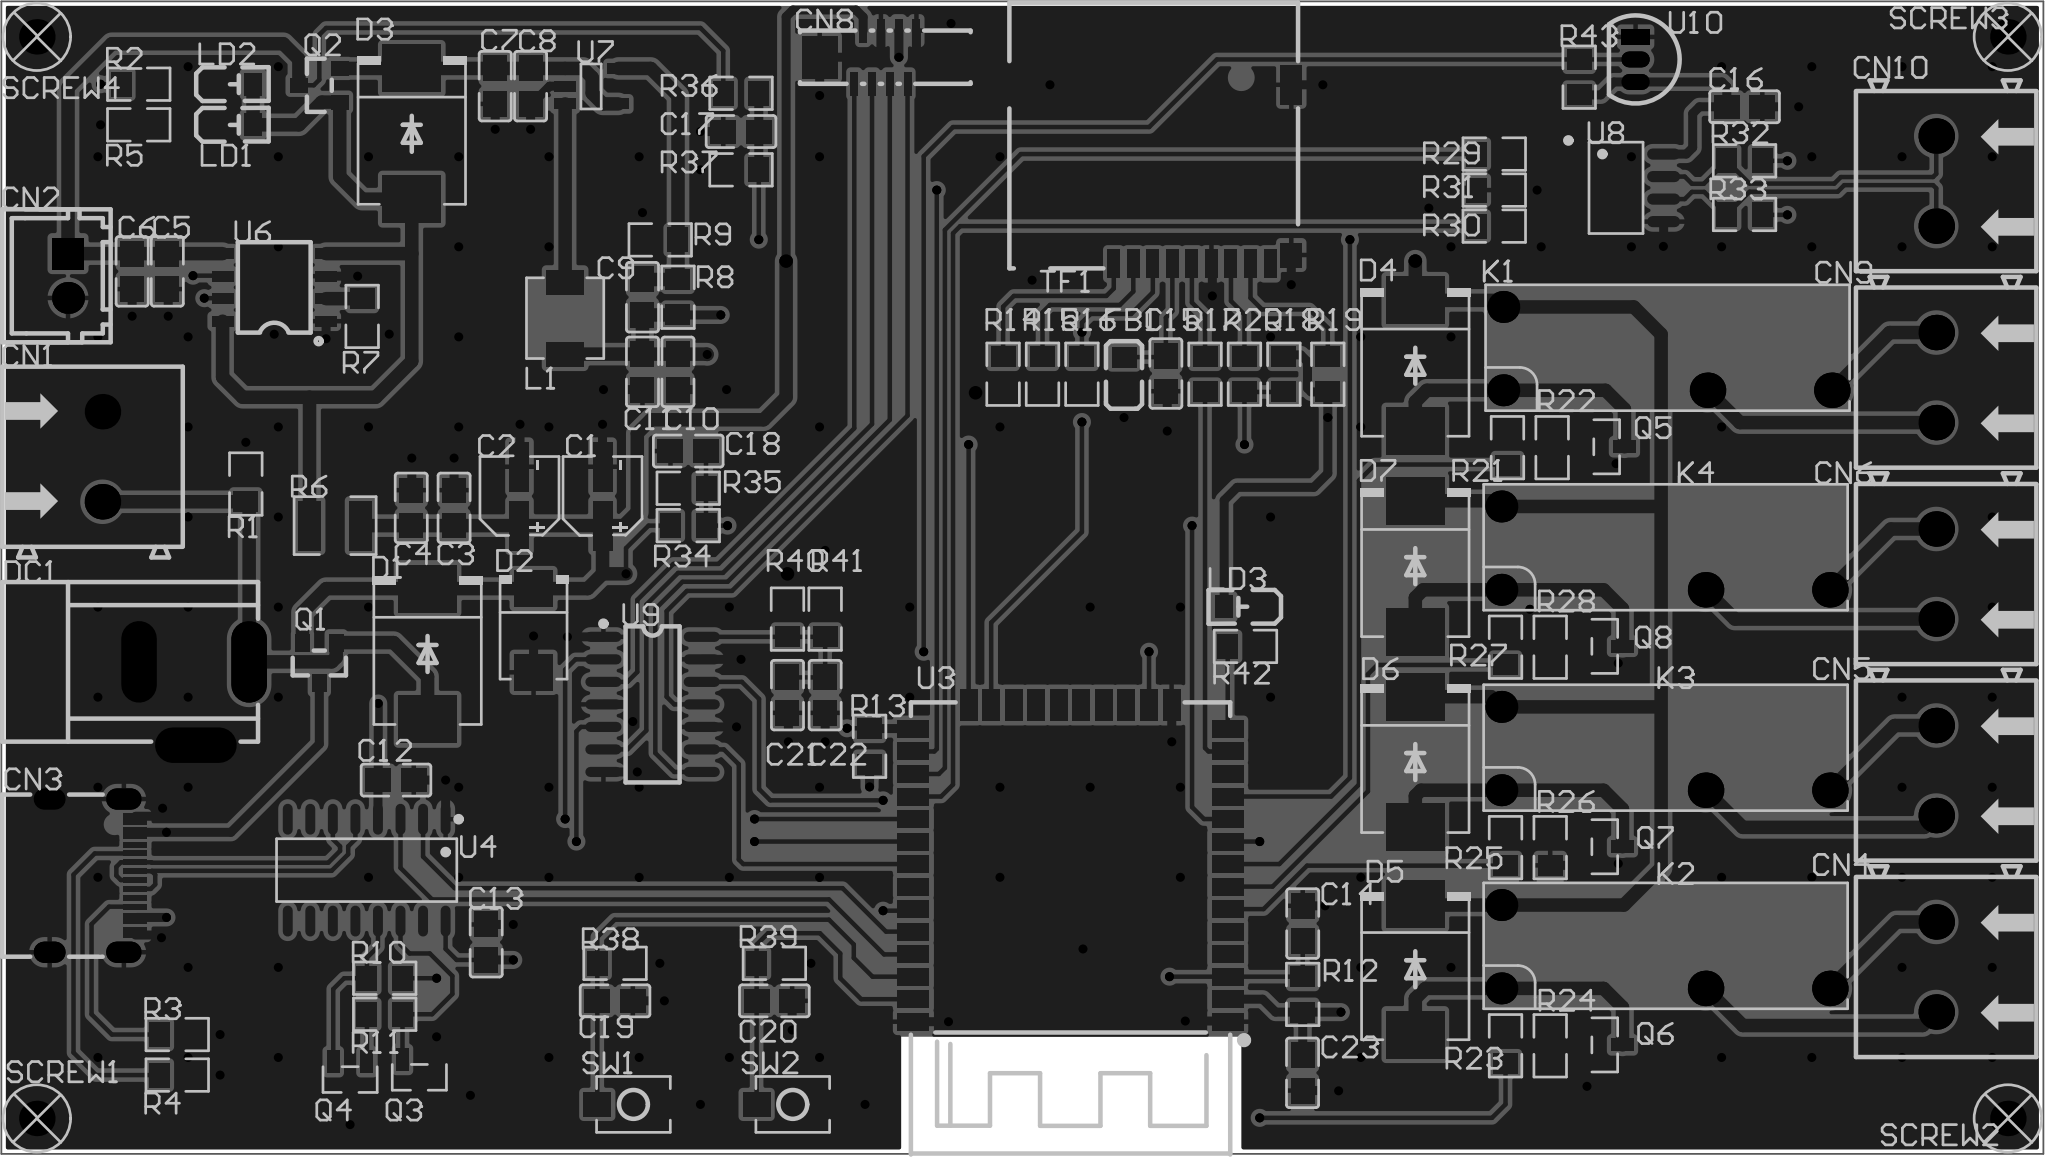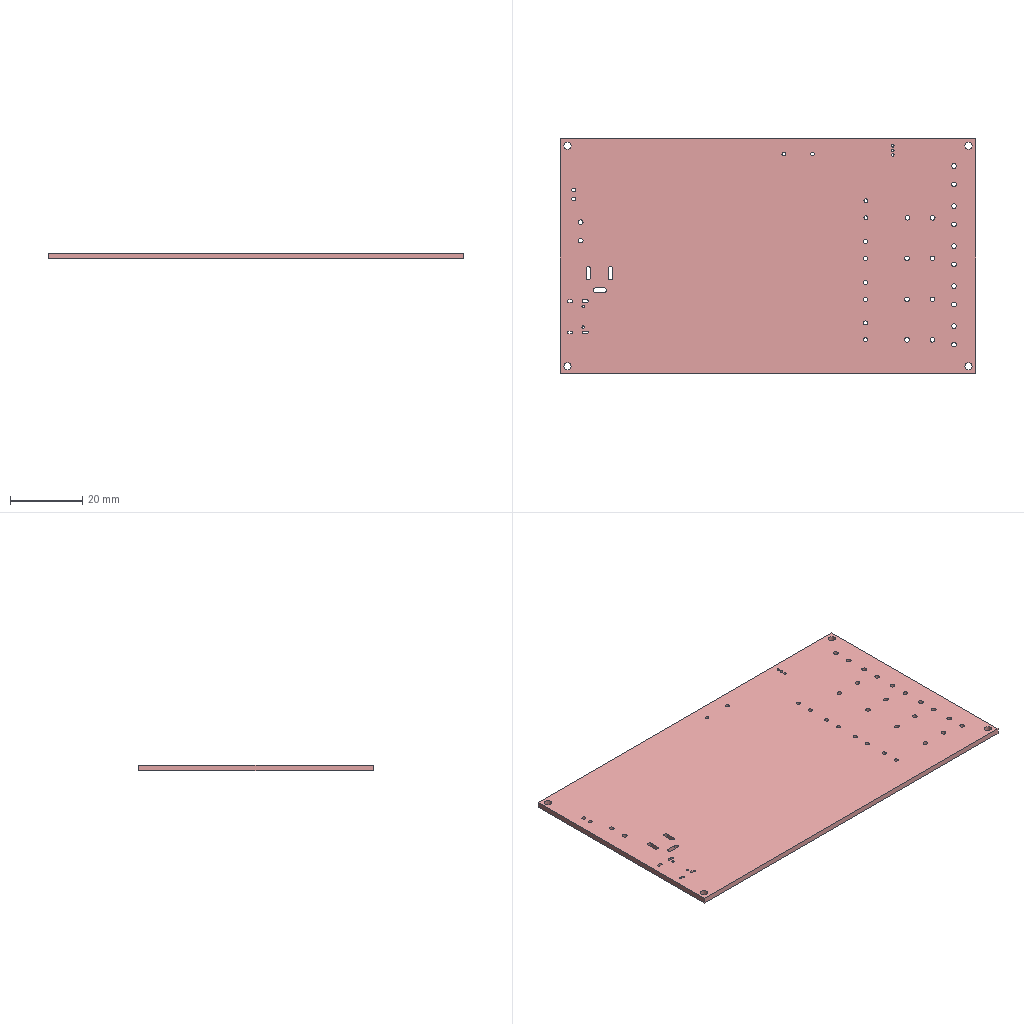Circuit board layout | Altium Designer | box 115 x 65 x 1.6 mm
Layer stack:
# Altium Designer layer stack of  (unit mm; dielectric type: 0 none, 1 core, 2 prepreg, 3 surface material)
index,name,kind,layer,copper_thickness_mm,dielectric_type,dielectric_thickness_mm,dielectric_material,dielectric_constant
0,Top Paste Mask Layer,other,,,,,,
1,Top Silkscreen Layer,other,,,,,,
2,Top Solder Mask Layer,dielectric,,,3,0.01,,3.3
3,Top Layer,copper,Top Layer,0.035,,,,
4,Dielectric1,dielectric,,,3,1.51,FR4,4.5
5,Bottom Layer,copper,Bottom Layer,0.035,,,,
6,Bottom Solder Mask Layer,dielectric,,,3,0.01,,3.3
7,Bottom Silkscreen Layer,other,,,,,,
8,Bottom Paste Mask Layer,other,,,,,,
# drill layer pairs: low layer,high layer
drill_pair,Top Layer,Bottom Layer
Part placement:
Designator,Comment,Layer,Footprint,Center-X(mm),Center-Y(mm),Rotation
C1,47uF,TopLayer,C_Ele_SMD_4x5.5mm,116.533,117.484,90
C2,47uF,TopLayer,C_Ele_SMD_4x5.5mm,111.856,117.484,90
C3,100nF,TopLayer,C0805,108.173,116.824,270
C4,10nF,TopLayer,C0805,105.76,116.824,270
C5,10uF,TopLayer,C0805,92.023,130.163,90
C6,10nF,TopLayer,C0805,90.043,130.163,90
C7,10uF,TopLayer,C0805,110.488,140.608,90
C8,10uF,TopLayer,C0805,112.482,140.608,90
C9,NF,TopLayer,C0805,118.783,128.705,90
C10,22uF,TopLayer,C0805,120.783,124.496,90
C11,22uF,TopLayer,C0805,118.783,124.496,90
C12,100nF,TopLayer,C0805,104.902,101.473,0
C13,100nF,TopLayer,C0805,109.982,92.329,270
C14,1uF,TopLayer,C0805,155.965,93.382,90
C15,10uF,TopLayer,C0805,148.258,124.403,270
C16,100nF,TopLayer,C0805,180.848,139.446,0
C17,100nF,TopLayer,C0805,124.333,138.049,180
C18,100nF,TopLayer,C0805,121.361,120.028,180
C19,100nF,TopLayer,C0805,117.239,89.023,180
C20,100nF,TopLayer,C0805,126.211,89.023,180
C21,100nF,TopLayer,C0805,126.949,106.264,90
C22,10nF,TopLayer,C0805,129.071,106.264,90
C23,100nF,TopLayer,C0805,155.956,84.963,270
CN1,,TopLayer,CONN-TH_2P-P5.00_WJ500V-5.08-2P,88.372,119.709,90
CN2,,TopLayer,CONN-TH_2P-P2.50_HX25003-2A,86.432,129.913,270
CN3,,TopLayer,USB_TYPE-C-16P,87.812,96.084,270
CN4,,TopLayer,CONN-TH_2P-P5.00_WJ500V-5.08-2P,191.643,90.932,270
CN5,,TopLayer,CONN-TH_2P-P5.00_WJ500V-5.08-2P,191.643,102.011,270
CN6,,TopLayer,CONN-TH_2P-P5.00_WJ500V-5.08-2P,191.643,113.094,270
CN8,,TopLayer,FPC-SMD_8P-P0.50_AFC11-S08ICC-00,132.461,142.24,0
CN9,,TopLayer,CONN-TH_2P-P5.00_WJ500V-5.08-2P,191.643,124.173,270
CN10,,TopLayer,CONN-TH_2P-P5.00_WJ500V-5.08-2P,191.643,135.255,270
D1,,TopLayer,SMC_L6.9-W5.9-LS7.9-RD,106.68,108.585,270
D2,,TopLayer,SMB_L4.6-W3.6-LS5.3-RD,112.649,109.911,270
D3,,TopLayer,SMC_L6.9-W5.9-LS7.9-RD,105.791,137.922,270
D4,,TopLayer,SMC_L6.9-W5.9-LS7.9-RD,162.306,124.841,270
D5,,TopLayer,SMC_L6.9-W5.9-LS7.9-RD,162.306,90.805,270
D6,,TopLayer,SMC_L6.9-W5.9-LS7.9-RD,162.306,102.489,270
D7,,TopLayer,SMC_L6.9-W5.9-LS7.9-RD,162.306,113.538,270
DC1,,TopLayer,DC-005_2.5,93.532,105.791,180
FB1,10uH,TopLayer,L0805,145.901,124.363,90
K1,,TopLayer,RELAY-TH_G5NB-1A-E-DCXX,176.512,125.807,0
K2,,TopLayer,RELAY-TH_G5NB-1A-E-DCXX,176.403,92.075,0
K3,,TopLayer,RELAY-TH_G5NB-1A-E-DCXX,176.403,103.251,0
K4,,TopLayer,RELAY-TH_G5NB-1A-E-DCXX,176.403,114.554,0
L1,2.2uH,TopLayer,IND-SMD_L4.4-W4.2,114.427,127.524,90
LD1,,TopLayer,LED_0805,95.75,138.429,0
LD2,,TopLayer,LED_0805,95.75,140.719,0
LD3,,TopLayer,LED_0805,152.641,111.247,180
Q1,,TopLayer,SOT-23_L2.9-W1.3-P1.90-LS2.4-BR,100.584,108.077,90
Q2,,TopLayer,SOT-23_L2.9-W1.3-P1.90-LS2.4-BR,100.584,140.658,0
Q3,,TopLayer,SOT-23-3_L2.9-W1.3-P1.90-LS2.4-BR,106.217,84.709,90
Q4,,TopLayer,SOT-23-3_L2.9-W1.3-P1.90-LS2.4-BR,102.317,84.582,90
Q5,,TopLayer,SOT-23-3_L2.9-W1.3-P1.90-LS2.4-BR,173.083,120.269,180
Q6,,TopLayer,SOT-23-3_L2.9-W1.3-P1.90-LS2.4-BR,172.974,86.537,180
Q7,,TopLayer,SOT-23-3_L2.9-W1.3-P1.90-LS2.4-BR,172.974,97.713,180
Q8,,TopLayer,SOT-23-3_L2.9-W1.3-P1.90-LS2.4-BR,172.974,109.016,180
R1,10K,TopLayer,R0805,96.445,118.169,270
R2,1.5K,TopLayer,R0805,90.416,140.719,0
R3,5.1K,TopLayer,R0805,92.583,87.122,180
R4,5.1K,TopLayer,R0805,92.583,84.836,180
R5,1.5K,TopLayer,R0805,90.416,138.429,0
R6,100mΩ,TopLayer,R1210,101.473,115.824,180
R7,1.5K,TopLayer,R0805,102.997,127.623,270
R8,180K,TopLayer,R0805,120.783,128.705,270
R9,40K,TopLayer,R0805,119.783,131.938,0
R10,1K,TopLayer,R0805,104.267,90.297,180
R11,1K,TopLayer,R0805,104.267,88.265,0
R12,10K,TopLayer,R0805,155.965,89.386,270
R13,10K,TopLayer,R0805,131.572,103.378,270
R14,2.2K,TopLayer,R0805,139.091,124.363,270
R15,2.2K,TopLayer,R0805,141.311,124.363,270
R16,10K,TopLayer,R0805,143.531,124.363,270
R17,10R,TopLayer,R0805,150.464,124.363,270
R18,2.2K,TopLayer,R0805,154.905,124.363,90
R19,2.2K,TopLayer,R0805,157.379,124.363,270
R20,220R,TopLayer,R0805,152.685,124.363,270
R21,4.7K,TopLayer,R0805,167.495,120.219,270
R22,4.7K,TopLayer,R0805,170.012,120.219,90
R23,4.7K,TopLayer,R0805,167.386,86.487,270
R24,4.7K,TopLayer,R0805,169.903,86.487,90
R25,4.7K,TopLayer,R0805,167.386,97.663,270
R26,4.7K,TopLayer,R0805,169.903,97.663,90
R27,4.7K,TopLayer,R0805,167.386,108.966,270
R28,4.7K,TopLayer,R0805,169.903,108.966,90
R29,300R,TopLayer,R0805,166.751,136.779,180
R30,300R,TopLayer,R0805,166.751,132.715,180
R31,10K,TopLayer,R0805,166.751,134.747,180
R32,120R,TopLayer,R0805,180.848,136.398,0
R33,0R,TopLayer,R0805,180.848,133.373,0
R34,100K,TopLayer,R0805,121.361,115.824,0
R35,100K,TopLayer,R0805,121.361,117.933,180
R36,100K,TopLayer,R0805,124.333,140.208,180
R37,100K,TopLayer,R0805,124.333,135.89,0
R38,10K,TopLayer,R0805,117.239,91.138,0
R39,10K,TopLayer,R0805,126.211,91.138,0
R40,0R,TopLayer,R0805,126.949,110.551,90
R41,0R,TopLayer,R0805,129.071,110.551,90
R42,1.5K,TopLayer,R0805,152.741,109.012,180
R43,4.7K,TopLayer,R0805,171.535,141.115,270
SCREW1,,TopLayer,M2螺丝,84.676,82.39,0
SCREW2,,TopLayer,M2螺丝,195.677,82.39,0
SCREW3,,TopLayer,M2螺丝,195.677,143.391,0
SCREW4,,TopLayer,M2螺丝,84.676,143.391,0
SW1,,TopLayer,Key_SMD_3x4x2,118.274,83.181,0
SW2,,TopLayer,Key_SMD_3x4x2,127.246,83.181,0
TF1,,TopLayer,TF-SMD_TF-CARD-H1.8,147.574,135.636,180
U3,,TopLayer,WIFIM-SMD_ESP-WROOM-32,142.891,96.776,180
U4,,TopLayer,SOP-16_L10.0-W3.9-P1.27-LS6.0-BL,103.251,96.393,180
U6,,TopLayer,ESOP-8_L4.9-W3.9-P1.27-LS6.0-BL-EP,98.045,129.258,90
U7,,TopLayer,SOT_XDC,115.927,140.608,0
U8,,TopLayer,SOP-8_L4.9-W3.9-P1.27-LS6.0-BL,173.609,134.874,270
U9,,TopLayer,SOIC-14_L8.6-W3.8-P1.27-LS6.0-BL,119.352,105.741,270
U10,,TopLayer,TO-92-3_L4.9-W3.7-P1.27-L,174.71,142.115,270
Pad and via stacks:
# Altium Designer via and pad stacks of  (unit mm). Each distinct definition once, with the count of objects using it.
# via: kind,start_layer,end_layer,hole_mm,diameter_mm,mode(0 simple;1 top-mid-bottom;2 full stack),diameter_per_layer,count,example_net
# pad: kind,layer,hole_mm,hole_type(0 round;1 square;2 slot),plating,top_size,top_shape(1 round;2 rect;3 octagon;9 rounded rect),mid_size,bottom_size,mode,footprint,size_per_layer,count,example
pad,Top Layer,0,0,plated,1.25x0.7,2,1.25x0.7,1.25x0.7,0,,,3,1
pad,Top Layer,0,0,plated,1.133x1.377,2,1.133x1.377,1.133x1.377,0,,,6,2
pad,Top Layer,0,0,plated,2.8x1.1,2,2.8x1.1,2.8x1.1,0,C_Ele_SMD_4x5.5mm,,4,C1.1
pad,Top Layer,0,0,plated,1.41x1.35,2,1.41x1.35,1.41x1.35,0,C0805,,42,C3.2
pad,Top Layer,0,0,plated,0.3x1.3,2,0.3x1.3,0.3x1.3,0,USB_TYPE-C-16P,,16,CN3.A1
pad,Top Layer,0,0,plated,0.4x1.35,2,0.4x1.35,0.4x1.35,0,FPC-SMD_8P-P0.50_AFC11-S08ICC-00,,8,CN8.1
pad,Top Layer,0,0,plated,2x2.4,2,2x2.4,2x2.4,0,FPC-SMD_8P-P0.50_AFC11-S08ICC-00,,2,CN8.9
pad,Top Layer,0,0,plated,2.7x3.3,2,2.7x3.3,2.7x3.3,0,SMC_L6.9-W5.9-LS7.9-RD,,12,D1.2
pad,Top Layer,0,0,plated,2.047x2.192,2,2.047x2.192,2.047x2.192,0,SMB_L4.6-W3.6-LS5.3-RD,,2,D2.2
pad,Top Layer,0,0,plated,1.133x1.377,2,1.133x1.377,1.133x1.377,0,L0805,,2,FB1.1
pad,Top Layer,0,0,plated,1.4x2.12,2,1.4x2.12,1.4x2.12,0,IND-SMD_L4.4-W4.2,,2,L1.1
pad,Top Layer,0,0,plated,1x1.25,2,1x1.25,1x1.25,0,LED_0805,,6,LD1.2
pad,Top Layer,0,0,plated,1x0.8,2,1x0.8,1x0.8,0,SOT-23_L2.9-W1.3-P1.90-LS2.4-BR,,6,Q1.2
pad,Top Layer,0,0,plated,1.25x0.7,2,1.25x0.7,1.25x0.7,0,SOT-23-3_L2.9-W1.3-P1.90-LS2.4-BR,,18,Q3.1
pad,Top Layer,0,0,plated,1.133x1.377,2,1.133x1.377,1.133x1.377,0,R0805,,84,R1.2
pad,Top Layer,0,0,plated,1.282x2.808,2,1.282x2.808,1.282x2.808,0,R1210,,2,R6.2
pad,Top Layer,0,0,plated,1.53x1.36,2,1.53x1.36,1.53x1.36,0,Key_SMD_3x4x2,,4,SW1.1
pad,Top Layer,0,0,plated,1.6x1.4,2,1.6x1.4,1.6x1.4,0,TF-SMD_TF-CARD-H1.8,,1,TF1.13
pad,Top Layer,0,0,plated,1.2x2.2,2,1.2x2.2,1.2x2.2,0,TF-SMD_TF-CARD-H1.8,,2,TF1.12
pad,Top Layer,0,0,plated,1.2x1.4,2,1.2x1.4,1.2x1.4,0,TF-SMD_TF-CARD-H1.8,,1,TF1.10
pad,Top Layer,0,0,plated,0.7x1.6,2,0.7x1.6,0.7x1.6,0,TF-SMD_TF-CARD-H1.8,,9,TF1.9
pad,Top Layer,0,0,plated,1.8x1.001,2,1.8x1.001,1.8x1.001,0,WIFIM-SMD_ESP-WROOM-32,,38,U3.4
pad,Top Layer,0,0,plated,4x4,2,4x4,4x4,0,WIFIM-SMD_ESP-WROOM-32,,1,U3.39
pad,Top Layer,0,0,plated,0.56x1.745,1,0.56x1.745,0.56x1.745,0,SOP-16_L10.0-W3.9-P1.27-LS6.0-BL,,16,U4.1
pad,Top Layer,0,0,plated,0.6x1.2,2,0.6x1.2,0.6x1.2,0,ESOP-8_L4.9-W3.9-P1.27-LS6.0-BL-EP,,8,U6.1
pad,Top Layer,0,0,plated,3.3x2.4,2,3.3x2.4,3.3x2.4,0,ESOP-8_L4.9-W3.9-P1.27-LS6.0-BL-EP,,1,U6.9
pad,Top Layer,0,0,plated,1.2x0.6,1,1.2x0.6,1.2x0.6,0,SOT_XDC,,1,U7.1
pad,Top Layer,0,0,plated,1.2x0.6,2,1.2x0.6,1.2x0.6,0,SOT_XDC,,4,U7.2
pad,Top Layer,0,0,plated,0.63x1.865,1,0.63x1.865,0.63x1.865,0,SOP-8_L4.9-W3.9-P1.27-LS6.0-BL,,8,U8.1
pad,Top Layer,0,0,plated,0.574x2.038,1,0.574x2.038,0.574x2.038,0,SOIC-14_L8.6-W3.8-P1.27-LS6.0-BL,,14,U9.8
pad,Multi-Layer,1.3,0,plated,2x2,1,2x2,2x2,0,CONN-TH_2P-P5.00_WJ500V-5.08-2P,,12,CN1.2
pad,Multi-Layer,1.1,0,plated,1.8x1.8,2,1.8x1.8,1.8x1.8,0,CONN-TH_2P-P2.50_HX25003-2A,,1,CN2.1
pad,Multi-Layer,1.1,0,plated,1.8x1.8,1,1.8x1.8,1.8x1.8,0,CONN-TH_2P-P2.50_HX25003-2A,,1,CN2.2
pad,Multi-Layer,0.7,2,plated,1.2x1.8,1,1.2x1.8,1.2x1.8,0,USB_TYPE-C-16P,,2,CN3.3
pad,Multi-Layer,0.7,2,plated,1.2x2,1,1.2x2,1.2x2,0,USB_TYPE-C-16P,,2,CN3.2
pad,Multi-Layer,1.2,2,plated,2x4.6,1,2x4.6,2x4.6,0,DC-005_2.5,,2,DC1.1
pad,Multi-Layer,1.2,2,plated,4.6x2,1,4.6x2,4.6x2,0,DC-005_2.5,,1,DC1.3
pad,Multi-Layer,1.1,0,plated,1.8x1.8,1,1.8x1.8,1.8x1.8,0,RELAY-TH_G5NB-1A-E-DCXX,,8,K1.4
pad,Multi-Layer,1.3,0,plated,2x2,1,2x2,2x2,0,RELAY-TH_G5NB-1A-E-DCXX,,8,K1.2
pad,Multi-Layer,2,0,plated,2x2,1,2x2,2x2,0,M2\u00C2\u00DD\u00CB\u00BF,,4,SCREW1.1
pad,Multi-Layer,0.7,0,plated,0.9x1.6,1,0.9x1.6,0.9x1.6,0,TO-92-3_L4.9-W3.7-P1.27-L,,2,U10.3
pad,Multi-Layer,0.7,0,plated,0.9x1.6,2,0.9x1.6,0.9x1.6,0,TO-92-3_L4.9-W3.7-P1.27-L,,1,U10.1
via,Top Layer,Bottom Layer,0.254,0.508,0,,213,$2N2545
via,Top Layer,Bottom Layer,0.381,0.762,0,,4,VEXT
Copper pours:
name,layer,net,type(0 solid;1 hatched;2 none)
Top Layer-GND,Top Layer,GND,0
Bottom Layer-GND,Bottom Layer,GND,0
Design rules, without the lines most boards share:
# Altium Designer design rules of  (exported by Altium Designer, unit mm)
# columns: name | kind | enabled | priority | scope1 | scope2 | descriptor | typed fields (field=value)
Plane_innerPlane | 0 | disabled | 2 | All | All | Clearance Constraint (Gap=8mil) (Disabled)(All),(All) | gap=0.2032
Copper_copperRegion | 0 | disabled | 3 | All | All | Clearance Constraint (Gap=8mil) (Disabled)(All),(All) | gap=0.2032
copperThickness1oz | 0 | enabled | 4 | All | All | Clearance Constraint (Gap=8mil) (All),(All) | gap=0.2032
copperThickness1oz_2 | 2 | enabled | 2 | All | All | Width Constraint (Min=8mil) (Max=100mil) (Preferred=8mil) (All) |
differentialPair | 51 | enabled | 1 | All | All | Differential Pairs Uncoupled Length using the Gap Constraints (Min=8mil) (Max=8mil) (Prefered=8mil)  and Width Constraints (Min=10mil) (Max=100mil) (Prefered=10mil) (All) |
viaSize | 11 | enabled | 1 | All | All | Routing Via (MinHoleWidth=10mil) (MaxHoleWidth=248.032mil) (PreferredHoleWidth=10mil) (MinWidth=20mil) (MaxWidth=393.701mil) (PreferedWidth=20mil) (All) | via_min_hole=0.254 via_max_hole=6.3 via_preferred_diameter=0.508 via_preferred_hole=0.254
solderMaskExpansion | 13 | enabled | 2 | All | All | Solder Mask Expansion (Expansion =2.008mil) (All) | expansion=0.051